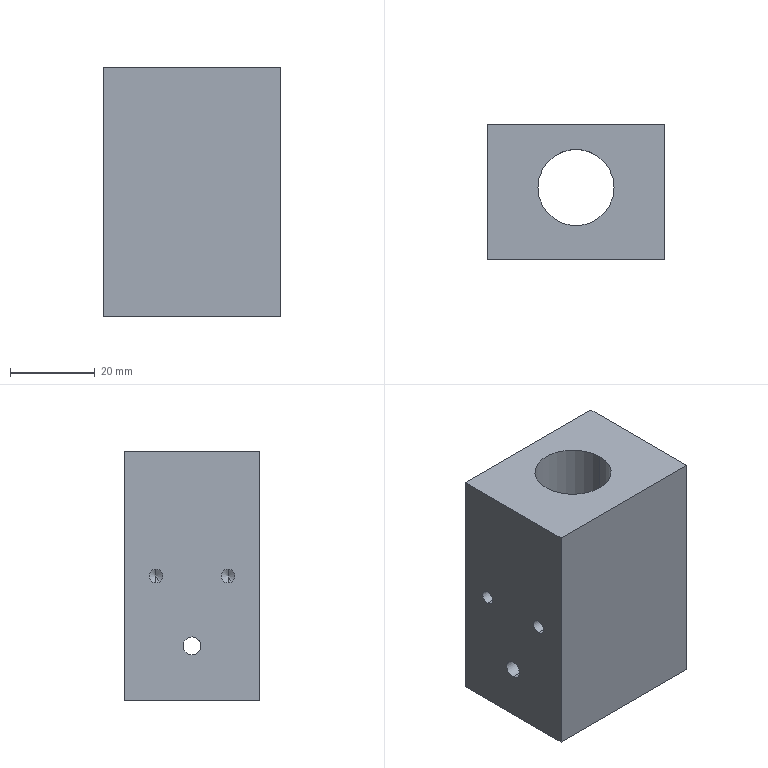Part | SolidWorks | features HoleWzd 3, ICE 2, Extrusion 1, MirrorPattern 1 | 1 solid | 71 faces | box 42 x 32 x 59 mm | volume 49987 mm3 | cylinder 40 | cone 16 | plane 15 | commonest cylinder face diameters 3.3 x16 3 x8 6 x8 4.2 x4 18 x2 27 x2